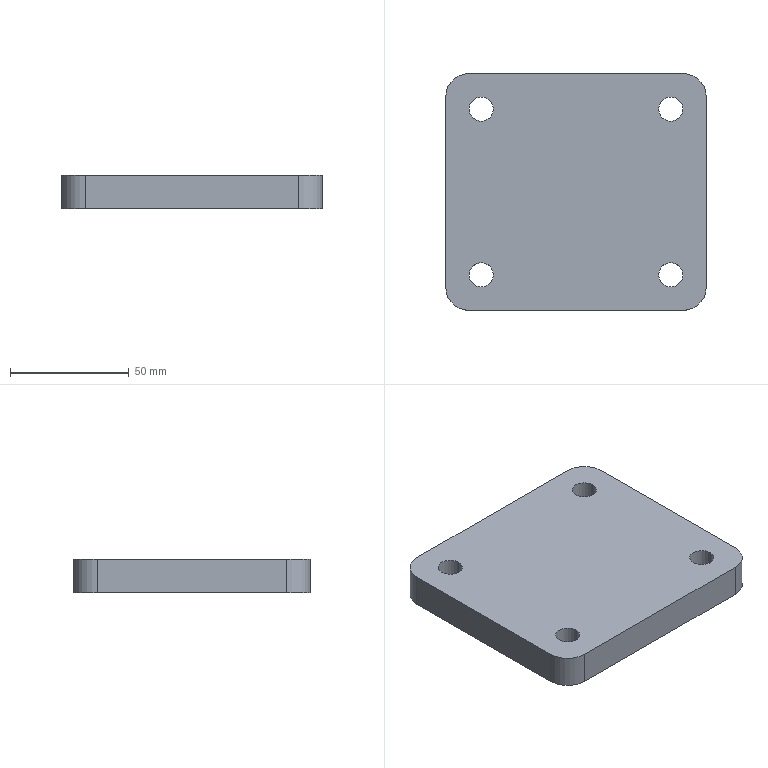Part | SolidWorks | features 3DProfileFeature 1, Extrusion 1, HoleWzd 1 | 1 solid | 18 faces | box 110 x 100 x 14 mm | volume 148222 mm3 | cylinder 12 | plane 6 | commonest cylinder face diameters 10.2 x8 20 x4
STEP:
#1=CARTESIAN_POINT('',(20.1,85.,0.));
#2=VERTEX_POINT('',#1);
#3=CARTESIAN_POINT('',(9.9,85.,0.));
#4=VERTEX_POINT('',#3);
#5=CARTESIAN_POINT('',(15.,85.,0.));
#6=DIRECTION('',(0.,0.,-1.));
#7=DIRECTION('',(-1.,0.,0.));
#8=AXIS2_PLACEMENT_3D('',#5,#6,#7);
#9=CIRCLE('',#8,5.1);
#10=EDGE_CURVE('',#2,#4,#9,.T.);
#11=ORIENTED_EDGE('',*,*,#10,.T.);
#12=CARTESIAN_POINT('',(9.9,85.,14.));
#13=VERTEX_POINT('',#12);
#14=CARTESIAN_POINT('',(9.9,85.,14.));
#15=DIRECTION('',(0.,0.,1.));
#16=VECTOR('',#15,1000.);
#17=LINE('',#14,#16);
#18=EDGE_CURVE('',#4,#13,#17,.T.);
#19=ORIENTED_EDGE('',*,*,#18,.T.);
#20=CARTESIAN_POINT('',(20.1,85.,14.));
#21=VERTEX_POINT('',#20);
#22=CARTESIAN_POINT('',(15.,85.,14.));
#23=DIRECTION('',(0.,0.,1.));
#24=DIRECTION('',(1.,0.,0.));
#25=AXIS2_PLACEMENT_3D('',#22,#23,#24);
#26=CIRCLE('',#25,5.1);
#27=EDGE_CURVE('',#13,#21,#26,.T.);
#28=ORIENTED_EDGE('',*,*,#27,.T.);
#29=CARTESIAN_POINT('',(20.1,85.,14.));
#30=DIRECTION('',(0.,0.,1.));
#31=VECTOR('',#30,1000.);
#32=LINE('',#29,#31);
#33=EDGE_CURVE('',#2,#21,#32,.T.);
#34=ORIENTED_EDGE('',*,*,#33,.F.);
#35=EDGE_LOOP('',(#11,#19,#28,#34));
#36=FACE_OUTER_BOUND('',#35,.T.);
#37=CARTESIAN_POINT('',(15.,85.,14.));
#38=DIRECTION('',(0.,0.,1.));
#39=DIRECTION('',(1.,0.,0.));
#40=AXIS2_PLACEMENT_3D('',#37,#38,#39);
#41=CYLINDRICAL_SURFACE('',#40,5.1);
#42=ADVANCED_FACE('',(#36),#41,.F.);
#43=CARTESIAN_POINT('',(100.1,85.,0.));
#44=VERTEX_POINT('',#43);
#45=CARTESIAN_POINT('',(89.9,85.,0.));
#46=VERTEX_POINT('',#45);
#47=CARTESIAN_POINT('',(95.,85.,0.));
#48=DIRECTION('',(0.,0.,-1.));
#49=DIRECTION('',(-1.,0.,0.));
#50=AXIS2_PLACEMENT_3D('',#47,#48,#49);
#51=CIRCLE('',#50,5.1);
#52=EDGE_CURVE('',#44,#46,#51,.T.);
#53=ORIENTED_EDGE('',*,*,#52,.T.);
#54=CARTESIAN_POINT('',(89.9,85.,14.));
#55=VERTEX_POINT('',#54);
#56=CARTESIAN_POINT('',(89.9,85.,14.));
#57=DIRECTION('',(0.,0.,1.));
#58=VECTOR('',#57,1000.);
#59=LINE('',#56,#58);
#60=EDGE_CURVE('',#46,#55,#59,.T.);
#61=ORIENTED_EDGE('',*,*,#60,.T.);
#62=CARTESIAN_POINT('',(100.1,85.,14.));
#63=VERTEX_POINT('',#62);
#64=CARTESIAN_POINT('',(95.,85.,14.));
#65=DIRECTION('',(0.,0.,1.));
#66=DIRECTION('',(1.,0.,0.));
#67=AXIS2_PLACEMENT_3D('',#64,#65,#66);
#68=CIRCLE('',#67,5.1);
#69=EDGE_CURVE('',#55,#63,#68,.T.);
#70=ORIENTED_EDGE('',*,*,#69,.T.);
#71=CARTESIAN_POINT('',(100.1,85.,14.));
#72=DIRECTION('',(0.,0.,1.));
#73=VECTOR('',#72,1000.);
#74=LINE('',#71,#73);
#75=EDGE_CURVE('',#44,#63,#74,.T.);
#76=ORIENTED_EDGE('',*,*,#75,.F.);
#77=EDGE_LOOP('',(#53,#61,#70,#76));
#78=FACE_OUTER_BOUND('',#77,.T.);
#79=CARTESIAN_POINT('',(95.,85.,14.));
#80=DIRECTION('',(0.,0.,1.));
#81=DIRECTION('',(1.,0.,0.));
#82=AXIS2_PLACEMENT_3D('',#79,#80,#81);
#83=CYLINDRICAL_SURFACE('',#82,5.1);
#84=ADVANCED_FACE('',(#78),#83,.F.);
#85=CARTESIAN_POINT('',(100.1,15.,0.));
#86=VERTEX_POINT('',#85);
#87=CARTESIAN_POINT('',(89.9,15.,0.));
#88=VERTEX_POINT('',#87);
#89=CARTESIAN_POINT('',(95.,15.,0.));
#90=DIRECTION('',(0.,0.,-1.));
#91=DIRECTION('',(-1.,0.,0.));
#92=AXIS2_PLACEMENT_3D('',#89,#90,#91);
#93=CIRCLE('',#92,5.1);
#94=EDGE_CURVE('',#86,#88,#93,.T.);
#95=ORIENTED_EDGE('',*,*,#94,.T.);
#96=CARTESIAN_POINT('',(89.9,15.,14.));
#97=VERTEX_POINT('',#96);
#98=CARTESIAN_POINT('',(89.9,15.,14.));
#99=DIRECTION('',(0.,0.,1.));
#100=VECTOR('',#99,1000.);
#101=LINE('',#98,#100);
#102=EDGE_CURVE('',#88,#97,#101,.T.);
#103=ORIENTED_EDGE('',*,*,#102,.T.);
#104=CARTESIAN_POINT('',(100.1,15.,14.));
#105=VERTEX_POINT('',#104);
#106=CARTESIAN_POINT('',(95.,15.,14.));
#107=DIRECTION('',(0.,0.,1.));
#108=DIRECTION('',(1.,0.,0.));
#109=AXIS2_PLACEMENT_3D('',#106,#107,#108);
#110=CIRCLE('',#109,5.1);
#111=EDGE_CURVE('',#97,#105,#110,.T.);
#112=ORIENTED_EDGE('',*,*,#111,.T.);
#113=CARTESIAN_POINT('',(100.1,15.,14.));
#114=DIRECTION('',(0.,0.,1.));
#115=VECTOR('',#114,1000.);
#116=LINE('',#113,#115);
#117=EDGE_CURVE('',#86,#105,#116,.T.);
#118=ORIENTED_EDGE('',*,*,#117,.F.);
#119=EDGE_LOOP('',(#95,#103,#112,#118));
#120=FACE_OUTER_BOUND('',#119,.T.);
#121=CARTESIAN_POINT('',(95.,15.,14.));
#122=DIRECTION('',(0.,0.,1.));
#123=DIRECTION('',(1.,0.,0.));
#124=AXIS2_PLACEMENT_3D('',#121,#122,#123);
#125=CYLINDRICAL_SURFACE('',#124,5.1);
#126=ADVANCED_FACE('',(#120),#125,.F.);
#127=CARTESIAN_POINT('',(20.1,15.,0.));
#128=VERTEX_POINT('',#127);
#129=CARTESIAN_POINT('',(9.9,15.,0.));
#130=VERTEX_POINT('',#129);
#131=CARTESIAN_POINT('',(15.,15.,0.));
#132=DIRECTION('',(0.,0.,-1.));
#133=DIRECTION('',(-1.,0.,0.));
#134=AXIS2_PLACEMENT_3D('',#131,#132,#133);
#135=CIRCLE('',#134,5.1);
#136=EDGE_CURVE('',#128,#130,#135,.T.);
#137=ORIENTED_EDGE('',*,*,#136,.T.);
#138=CARTESIAN_POINT('',(9.9,15.,14.));
#139=VERTEX_POINT('',#138);
#140=CARTESIAN_POINT('',(9.9,15.,14.));
#141=DIRECTION('',(0.,0.,1.));
#142=VECTOR('',#141,1000.);
#143=LINE('',#140,#142);
#144=EDGE_CURVE('',#130,#139,#143,.T.);
#145=ORIENTED_EDGE('',*,*,#144,.T.);
#146=CARTESIAN_POINT('',(20.1,15.,14.));
#147=VERTEX_POINT('',#146);
#148=CARTESIAN_POINT('',(15.,15.,14.));
#149=DIRECTION('',(0.,0.,1.));
#150=DIRECTION('',(1.,0.,0.));
#151=AXIS2_PLACEMENT_3D('',#148,#149,#150);
#152=CIRCLE('',#151,5.1);
#153=EDGE_CURVE('',#139,#147,#152,.T.);
#154=ORIENTED_EDGE('',*,*,#153,.T.);
#155=CARTESIAN_POINT('',(20.1,15.,14.));
#156=DIRECTION('',(0.,0.,1.));
#157=VECTOR('',#156,1000.);
#158=LINE('',#155,#157);
#159=EDGE_CURVE('',#128,#147,#158,.T.);
#160=ORIENTED_EDGE('',*,*,#159,.F.);
#161=EDGE_LOOP('',(#137,#145,#154,#160));
#162=FACE_OUTER_BOUND('',#161,.T.);
#163=CARTESIAN_POINT('',(15.,15.,14.));
#164=DIRECTION('',(0.,0.,1.));
#165=DIRECTION('',(1.,0.,0.));
#166=AXIS2_PLACEMENT_3D('',#163,#164,#165);
#167=CYLINDRICAL_SURFACE('',#166,5.1);
#168=ADVANCED_FACE('',(#162),#167,.F.);
#169=CARTESIAN_POINT('',(0.,10.,0.));
#170=VERTEX_POINT('',#169);
#171=CARTESIAN_POINT('',(10.,0.,0.));
#172=VERTEX_POINT('',#171);
#173=CARTESIAN_POINT('',(10.,10.,0.));
#174=DIRECTION('',(0.,0.,1.));
#175=DIRECTION('',(-1.,0.,0.));
#176=AXIS2_PLACEMENT_3D('',#173,#174,#175);
#177=CIRCLE('',#176,10.);
#178=EDGE_CURVE('',#170,#172,#177,.T.);
#179=ORIENTED_EDGE('',*,*,#178,.T.);
#180=CARTESIAN_POINT('',(10.,0.,14.));
#181=VERTEX_POINT('',#180);
#182=CARTESIAN_POINT('',(10.,0.,14.));
#183=DIRECTION('',(0.,0.,-1.));
#184=VECTOR('',#183,1000.);
#185=LINE('',#182,#184);
#186=EDGE_CURVE('',#181,#172,#185,.T.);
#187=ORIENTED_EDGE('',*,*,#186,.F.);
#188=CARTESIAN_POINT('',(0.,10.,14.));
#189=VERTEX_POINT('',#188);
#190=CARTESIAN_POINT('',(10.,10.,14.));
#191=DIRECTION('',(0.,0.,1.));
#192=DIRECTION('',(-1.,0.,0.));
#193=AXIS2_PLACEMENT_3D('',#190,#191,#192);
#194=CIRCLE('',#193,10.);
#195=EDGE_CURVE('',#189,#181,#194,.T.);
#196=ORIENTED_EDGE('',*,*,#195,.F.);
#197=CARTESIAN_POINT('',(0.,10.,14.));
#198=DIRECTION('',(0.,0.,-1.));
#199=VECTOR('',#198,1000.);
#200=LINE('',#197,#199);
#201=EDGE_CURVE('',#189,#170,#200,.T.);
#202=ORIENTED_EDGE('',*,*,#201,.T.);
#203=EDGE_LOOP('',(#179,#187,#196,#202));
#204=FACE_OUTER_BOUND('',#203,.T.);
#205=CARTESIAN_POINT('',(10.,10.,14.));
#206=DIRECTION('',(0.,0.,-1.));
#207=DIRECTION('',(-1.,0.,0.));
#208=AXIS2_PLACEMENT_3D('',#205,#206,#207);
#209=CYLINDRICAL_SURFACE('',#208,10.);
#210=ADVANCED_FACE('',(#204),#209,.T.);
#211=CARTESIAN_POINT('',(100.,0.,0.));
#212=VERTEX_POINT('',#211);
#213=CARTESIAN_POINT('',(10.,0.,0.));
#214=DIRECTION('',(1.,0.,0.));
#215=VECTOR('',#214,1000.);
#216=LINE('',#213,#215);
#217=EDGE_CURVE('',#172,#212,#216,.T.);
#218=ORIENTED_EDGE('',*,*,#217,.T.);
#219=CARTESIAN_POINT('',(100.,0.,14.));
#220=VERTEX_POINT('',#219);
#221=CARTESIAN_POINT('',(100.,0.,14.));
#222=DIRECTION('',(0.,0.,-1.));
#223=VECTOR('',#222,1000.);
#224=LINE('',#221,#223);
#225=EDGE_CURVE('',#220,#212,#224,.T.);
#226=ORIENTED_EDGE('',*,*,#225,.F.);
#227=CARTESIAN_POINT('',(10.,0.,14.));
#228=DIRECTION('',(1.,0.,0.));
#229=VECTOR('',#228,1000.);
#230=LINE('',#227,#229);
#231=EDGE_CURVE('',#181,#220,#230,.T.);
#232=ORIENTED_EDGE('',*,*,#231,.F.);
#233=ORIENTED_EDGE('',*,*,#186,.T.);
#234=EDGE_LOOP('',(#218,#226,#232,#233));
#235=FACE_OUTER_BOUND('',#234,.T.);
#236=CARTESIAN_POINT('',(10.,0.,14.));
#237=DIRECTION('',(0.,1.,0.));
#238=DIRECTION('',(0.,0.,1.));
#239=AXIS2_PLACEMENT_3D('',#236,#237,#238);
#240=PLANE('',#239);
#241=ADVANCED_FACE('',(#235),#240,.F.);
#242=CARTESIAN_POINT('',(110.,10.,0.));
#243=VERTEX_POINT('',#242);
#244=CARTESIAN_POINT('',(100.,10.,0.));
#245=DIRECTION('',(0.,0.,1.));
#246=DIRECTION('',(1.,0.,0.));
#247=AXIS2_PLACEMENT_3D('',#244,#245,#246);
#248=CIRCLE('',#247,10.);
#249=EDGE_CURVE('',#212,#243,#248,.T.);
#250=ORIENTED_EDGE('',*,*,#249,.T.);
#251=CARTESIAN_POINT('',(110.,10.,14.));
#252=VERTEX_POINT('',#251);
#253=CARTESIAN_POINT('',(110.,10.,14.));
#254=DIRECTION('',(0.,0.,-1.));
#255=VECTOR('',#254,1000.);
#256=LINE('',#253,#255);
#257=EDGE_CURVE('',#252,#243,#256,.T.);
#258=ORIENTED_EDGE('',*,*,#257,.F.);
#259=CARTESIAN_POINT('',(100.,10.,14.));
#260=DIRECTION('',(0.,0.,1.));
#261=DIRECTION('',(1.,0.,0.));
#262=AXIS2_PLACEMENT_3D('',#259,#260,#261);
#263=CIRCLE('',#262,10.);
#264=EDGE_CURVE('',#220,#252,#263,.T.);
#265=ORIENTED_EDGE('',*,*,#264,.F.);
#266=ORIENTED_EDGE('',*,*,#225,.T.);
#267=EDGE_LOOP('',(#250,#258,#265,#266));
#268=FACE_OUTER_BOUND('',#267,.T.);
#269=CARTESIAN_POINT('',(100.,10.,14.));
#270=DIRECTION('',(0.,0.,-1.));
#271=DIRECTION('',(-1.,0.,0.));
#272=AXIS2_PLACEMENT_3D('',#269,#270,#271);
#273=CYLINDRICAL_SURFACE('',#272,10.);
#274=ADVANCED_FACE('',(#268),#273,.T.);
#275=CARTESIAN_POINT('',(110.,90.,0.));
#276=VERTEX_POINT('',#275);
#277=CARTESIAN_POINT('',(110.,10.,0.));
#278=DIRECTION('',(0.,1.,0.));
#279=VECTOR('',#278,1000.);
#280=LINE('',#277,#279);
#281=EDGE_CURVE('',#243,#276,#280,.T.);
#282=ORIENTED_EDGE('',*,*,#281,.T.);
#283=CARTESIAN_POINT('',(110.,90.,14.));
#284=VERTEX_POINT('',#283);
#285=CARTESIAN_POINT('',(110.,90.,14.));
#286=DIRECTION('',(0.,0.,-1.));
#287=VECTOR('',#286,1000.);
#288=LINE('',#285,#287);
#289=EDGE_CURVE('',#284,#276,#288,.T.);
#290=ORIENTED_EDGE('',*,*,#289,.F.);
#291=CARTESIAN_POINT('',(110.,10.,14.));
#292=DIRECTION('',(0.,1.,0.));
#293=VECTOR('',#292,1000.);
#294=LINE('',#291,#293);
#295=EDGE_CURVE('',#252,#284,#294,.T.);
#296=ORIENTED_EDGE('',*,*,#295,.F.);
#297=ORIENTED_EDGE('',*,*,#257,.T.);
#298=EDGE_LOOP('',(#282,#290,#296,#297));
#299=FACE_OUTER_BOUND('',#298,.T.);
#300=CARTESIAN_POINT('',(110.,10.,14.));
#301=DIRECTION('',(-1.,0.,0.));
#302=DIRECTION('',(0.,0.,1.));
#303=AXIS2_PLACEMENT_3D('',#300,#301,#302);
#304=PLANE('',#303);
#305=ADVANCED_FACE('',(#299),#304,.F.);
#306=CARTESIAN_POINT('',(100.,100.,0.));
#307=VERTEX_POINT('',#306);
#308=CARTESIAN_POINT('',(100.,90.,0.));
#309=DIRECTION('',(0.,0.,1.));
#310=DIRECTION('',(-1.,0.,0.));
#311=AXIS2_PLACEMENT_3D('',#308,#309,#310);
#312=CIRCLE('',#311,10.);
#313=EDGE_CURVE('',#276,#307,#312,.T.);
#314=ORIENTED_EDGE('',*,*,#313,.T.);
#315=CARTESIAN_POINT('',(100.,100.,14.));
#316=VERTEX_POINT('',#315);
#317=CARTESIAN_POINT('',(100.,100.,14.));
#318=DIRECTION('',(0.,0.,-1.));
#319=VECTOR('',#318,1000.);
#320=LINE('',#317,#319);
#321=EDGE_CURVE('',#316,#307,#320,.T.);
#322=ORIENTED_EDGE('',*,*,#321,.F.);
#323=CARTESIAN_POINT('',(100.,90.,14.));
#324=DIRECTION('',(0.,0.,1.));
#325=DIRECTION('',(-1.,0.,0.));
#326=AXIS2_PLACEMENT_3D('',#323,#324,#325);
#327=CIRCLE('',#326,10.);
#328=EDGE_CURVE('',#284,#316,#327,.T.);
#329=ORIENTED_EDGE('',*,*,#328,.F.);
#330=ORIENTED_EDGE('',*,*,#289,.T.);
#331=EDGE_LOOP('',(#314,#322,#329,#330));
#332=FACE_OUTER_BOUND('',#331,.T.);
#333=CARTESIAN_POINT('',(100.,90.,14.));
#334=DIRECTION('',(0.,0.,-1.));
#335=DIRECTION('',(-1.,0.,0.));
#336=AXIS2_PLACEMENT_3D('',#333,#334,#335);
#337=CYLINDRICAL_SURFACE('',#336,10.);
#338=ADVANCED_FACE('',(#332),#337,.T.);
#339=CARTESIAN_POINT('',(10.,100.,0.));
#340=VERTEX_POINT('',#339);
#341=CARTESIAN_POINT('',(10.,100.,0.));
#342=DIRECTION('',(-1.,0.,0.));
#343=VECTOR('',#342,1000.);
#344=LINE('',#341,#343);
#345=EDGE_CURVE('',#307,#340,#344,.T.);
#346=ORIENTED_EDGE('',*,*,#345,.T.);
#347=CARTESIAN_POINT('',(10.,100.,14.));
#348=VERTEX_POINT('',#347);
#349=CARTESIAN_POINT('',(10.,100.,14.));
#350=DIRECTION('',(0.,0.,-1.));
#351=VECTOR('',#350,1000.);
#352=LINE('',#349,#351);
#353=EDGE_CURVE('',#348,#340,#352,.T.);
#354=ORIENTED_EDGE('',*,*,#353,.F.);
#355=CARTESIAN_POINT('',(10.,100.,14.));
#356=DIRECTION('',(-1.,0.,0.));
#357=VECTOR('',#356,1000.);
#358=LINE('',#355,#357);
#359=EDGE_CURVE('',#316,#348,#358,.T.);
#360=ORIENTED_EDGE('',*,*,#359,.F.);
#361=ORIENTED_EDGE('',*,*,#321,.T.);
#362=EDGE_LOOP('',(#346,#354,#360,#361));
#363=FACE_OUTER_BOUND('',#362,.T.);
#364=CARTESIAN_POINT('',(10.,100.,14.));
#365=DIRECTION('',(0.,-1.,0.));
#366=DIRECTION('',(0.,0.,-1.));
#367=AXIS2_PLACEMENT_3D('',#364,#365,#366);
#368=PLANE('',#367);
#369=ADVANCED_FACE('',(#363),#368,.F.);
#370=CARTESIAN_POINT('',(0.,90.,0.));
#371=VERTEX_POINT('',#370);
#372=CARTESIAN_POINT('',(10.,90.,0.));
#373=DIRECTION('',(0.,0.,1.));
#374=DIRECTION('',(-1.,0.,0.));
#375=AXIS2_PLACEMENT_3D('',#372,#373,#374);
#376=CIRCLE('',#375,10.);
#377=EDGE_CURVE('',#340,#371,#376,.T.);
#378=ORIENTED_EDGE('',*,*,#377,.T.);
#379=CARTESIAN_POINT('',(0.,90.,14.));
#380=VERTEX_POINT('',#379);
#381=CARTESIAN_POINT('',(0.,90.,14.));
#382=DIRECTION('',(0.,0.,-1.));
#383=VECTOR('',#382,1000.);
#384=LINE('',#381,#383);
#385=EDGE_CURVE('',#380,#371,#384,.T.);
#386=ORIENTED_EDGE('',*,*,#385,.F.);
#387=CARTESIAN_POINT('',(10.,90.,14.));
#388=DIRECTION('',(0.,0.,1.));
#389=DIRECTION('',(-1.,0.,0.));
#390=AXIS2_PLACEMENT_3D('',#387,#388,#389);
#391=CIRCLE('',#390,10.);
#392=EDGE_CURVE('',#348,#380,#391,.T.);
#393=ORIENTED_EDGE('',*,*,#392,.F.);
#394=ORIENTED_EDGE('',*,*,#353,.T.);
#395=EDGE_LOOP('',(#378,#386,#393,#394));
#396=FACE_OUTER_BOUND('',#395,.T.);
#397=CARTESIAN_POINT('',(10.,90.,14.));
#398=DIRECTION('',(0.,0.,-1.));
#399=DIRECTION('',(-1.,0.,0.));
#400=AXIS2_PLACEMENT_3D('',#397,#398,#399);
#401=CYLINDRICAL_SURFACE('',#400,10.);
#402=ADVANCED_FACE('',(#396),#401,.T.);
#403=CARTESIAN_POINT('',(0.,10.,0.));
#404=DIRECTION('',(0.,-1.,0.));
#405=VECTOR('',#404,1000.);
#406=LINE('',#403,#405);
#407=EDGE_CURVE('',#371,#170,#406,.T.);
#408=ORIENTED_EDGE('',*,*,#407,.T.);
#409=ORIENTED_EDGE('',*,*,#201,.F.);
#410=CARTESIAN_POINT('',(0.,10.,14.));
#411=DIRECTION('',(0.,-1.,0.));
#412=VECTOR('',#411,1000.);
#413=LINE('',#410,#412);
#414=EDGE_CURVE('',#380,#189,#413,.T.);
#415=ORIENTED_EDGE('',*,*,#414,.F.);
#416=ORIENTED_EDGE('',*,*,#385,.T.);
#417=EDGE_LOOP('',(#408,#409,#415,#416));
#418=FACE_OUTER_BOUND('',#417,.T.);
#419=CARTESIAN_POINT('',(0.,10.,14.));
#420=DIRECTION('',(1.,0.,0.));
#421=DIRECTION('',(0.,0.,-1.));
#422=AXIS2_PLACEMENT_3D('',#419,#420,#421);
#423=PLANE('',#422);
#424=ADVANCED_FACE('',(#418),#423,.F.);
#425=CARTESIAN_POINT('',(15.,85.,14.));
#426=DIRECTION('',(0.,0.,1.));
#427=DIRECTION('',(1.,0.,0.));
#428=AXIS2_PLACEMENT_3D('',#425,#426,#427);
#429=CIRCLE('',#428,5.1);
#430=EDGE_CURVE('',#21,#13,#429,.T.);
#431=ORIENTED_EDGE('',*,*,#430,.F.);
#432=ORIENTED_EDGE('',*,*,#27,.F.);
#433=EDGE_LOOP('',(#431,#432));
#434=FACE_BOUND('',#433,.T.);
#435=CARTESIAN_POINT('',(95.,85.,14.));
#436=DIRECTION('',(0.,0.,1.));
#437=DIRECTION('',(1.,0.,0.));
#438=AXIS2_PLACEMENT_3D('',#435,#436,#437);
#439=CIRCLE('',#438,5.1);
#440=EDGE_CURVE('',#63,#55,#439,.T.);
#441=ORIENTED_EDGE('',*,*,#440,.F.);
#442=ORIENTED_EDGE('',*,*,#69,.F.);
#443=EDGE_LOOP('',(#441,#442));
#444=FACE_BOUND('',#443,.T.);
#445=CARTESIAN_POINT('',(95.,15.,14.));
#446=DIRECTION('',(0.,0.,1.));
#447=DIRECTION('',(1.,0.,0.));
#448=AXIS2_PLACEMENT_3D('',#445,#446,#447);
#449=CIRCLE('',#448,5.1);
#450=EDGE_CURVE('',#105,#97,#449,.T.);
#451=ORIENTED_EDGE('',*,*,#450,.F.);
#452=ORIENTED_EDGE('',*,*,#111,.F.);
#453=EDGE_LOOP('',(#451,#452));
#454=FACE_BOUND('',#453,.T.);
#455=CARTESIAN_POINT('',(15.,15.,14.));
#456=DIRECTION('',(0.,0.,1.));
#457=DIRECTION('',(1.,0.,0.));
#458=AXIS2_PLACEMENT_3D('',#455,#456,#457);
#459=CIRCLE('',#458,5.1);
#460=EDGE_CURVE('',#147,#139,#459,.T.);
#461=ORIENTED_EDGE('',*,*,#460,.F.);
#462=ORIENTED_EDGE('',*,*,#153,.F.);
#463=EDGE_LOOP('',(#461,#462));
#464=FACE_BOUND('',#463,.T.);
#465=ORIENTED_EDGE('',*,*,#195,.T.);
#466=ORIENTED_EDGE('',*,*,#231,.T.);
#467=ORIENTED_EDGE('',*,*,#264,.T.);
#468=ORIENTED_EDGE('',*,*,#295,.T.);
#469=ORIENTED_EDGE('',*,*,#328,.T.);
#470=ORIENTED_EDGE('',*,*,#359,.T.);
#471=ORIENTED_EDGE('',*,*,#392,.T.);
#472=ORIENTED_EDGE('',*,*,#414,.T.);
#473=EDGE_LOOP('',(#465,#466,#467,#468,#469,#470,#471,#472));
#474=FACE_OUTER_BOUND('',#473,.T.);
#475=CARTESIAN_POINT('',(10.,10.,14.));
#476=DIRECTION('',(0.,0.,-1.));
#477=DIRECTION('',(-1.,0.,0.));
#478=AXIS2_PLACEMENT_3D('',#475,#476,#477);
#479=PLANE('',#478);
#480=ADVANCED_FACE('',(#434,#444,#454,#464,#474),#479,.F.);
#481=ORIENTED_EDGE('',*,*,#10,.F.);
#482=CARTESIAN_POINT('',(15.,85.,0.));
#483=DIRECTION('',(0.,0.,-1.));
#484=DIRECTION('',(-1.,0.,0.));
#485=AXIS2_PLACEMENT_3D('',#482,#483,#484);
#486=CIRCLE('',#485,5.1);
#487=EDGE_CURVE('',#4,#2,#486,.T.);
#488=ORIENTED_EDGE('',*,*,#487,.F.);
#489=EDGE_LOOP('',(#481,#488));
#490=FACE_BOUND('',#489,.T.);
#491=ORIENTED_EDGE('',*,*,#52,.F.);
#492=CARTESIAN_POINT('',(95.,85.,0.));
#493=DIRECTION('',(0.,0.,-1.));
#494=DIRECTION('',(-1.,0.,0.));
#495=AXIS2_PLACEMENT_3D('',#492,#493,#494);
#496=CIRCLE('',#495,5.1);
#497=EDGE_CURVE('',#46,#44,#496,.T.);
#498=ORIENTED_EDGE('',*,*,#497,.F.);
#499=EDGE_LOOP('',(#491,#498));
#500=FACE_BOUND('',#499,.T.);
#501=ORIENTED_EDGE('',*,*,#94,.F.);
#502=CARTESIAN_POINT('',(95.,15.,0.));
#503=DIRECTION('',(0.,0.,-1.));
#504=DIRECTION('',(-1.,0.,0.));
#505=AXIS2_PLACEMENT_3D('',#502,#503,#504);
#506=CIRCLE('',#505,5.1);
#507=EDGE_CURVE('',#88,#86,#506,.T.);
#508=ORIENTED_EDGE('',*,*,#507,.F.);
#509=EDGE_LOOP('',(#501,#508));
#510=FACE_BOUND('',#509,.T.);
#511=ORIENTED_EDGE('',*,*,#136,.F.);
#512=CARTESIAN_POINT('',(15.,15.,0.));
#513=DIRECTION('',(0.,0.,-1.));
#514=DIRECTION('',(-1.,0.,0.));
#515=AXIS2_PLACEMENT_3D('',#512,#513,#514);
#516=CIRCLE('',#515,5.1);
#517=EDGE_CURVE('',#130,#128,#516,.T.);
#518=ORIENTED_EDGE('',*,*,#517,.F.);
#519=EDGE_LOOP('',(#511,#518));
#520=FACE_BOUND('',#519,.T.);
#521=ORIENTED_EDGE('',*,*,#178,.F.);
#522=ORIENTED_EDGE('',*,*,#407,.F.);
#523=ORIENTED_EDGE('',*,*,#377,.F.);
#524=ORIENTED_EDGE('',*,*,#345,.F.);
#525=ORIENTED_EDGE('',*,*,#313,.F.);
#526=ORIENTED_EDGE('',*,*,#281,.F.);
#527=ORIENTED_EDGE('',*,*,#249,.F.);
#528=ORIENTED_EDGE('',*,*,#217,.F.);
#529=EDGE_LOOP('',(#521,#522,#523,#524,#525,#526,#527,#528));
#530=FACE_OUTER_BOUND('',#529,.T.);
#531=CARTESIAN_POINT('',(10.,10.,0.));
#532=DIRECTION('',(0.,0.,-1.));
#533=DIRECTION('',(-1.,0.,0.));
#534=AXIS2_PLACEMENT_3D('',#531,#532,#533);
#535=PLANE('',#534);
#536=ADVANCED_FACE('',(#490,#500,#510,#520,#530),#535,.T.);
#537=ORIENTED_EDGE('',*,*,#144,.F.);
#538=ORIENTED_EDGE('',*,*,#517,.T.);
#539=ORIENTED_EDGE('',*,*,#159,.T.);
#540=ORIENTED_EDGE('',*,*,#460,.T.);
#541=EDGE_LOOP('',(#537,#538,#539,#540));
#542=FACE_OUTER_BOUND('',#541,.T.);
#543=CARTESIAN_POINT('',(15.,15.,14.));
#544=DIRECTION('',(0.,0.,1.));
#545=DIRECTION('',(1.,0.,0.));
#546=AXIS2_PLACEMENT_3D('',#543,#544,#545);
#547=CYLINDRICAL_SURFACE('',#546,5.1);
#548=ADVANCED_FACE('',(#542),#547,.F.);
#549=ORIENTED_EDGE('',*,*,#102,.F.);
#550=ORIENTED_EDGE('',*,*,#507,.T.);
#551=ORIENTED_EDGE('',*,*,#117,.T.);
#552=ORIENTED_EDGE('',*,*,#450,.T.);
#553=EDGE_LOOP('',(#549,#550,#551,#552));
#554=FACE_OUTER_BOUND('',#553,.T.);
#555=CARTESIAN_POINT('',(95.,15.,14.));
#556=DIRECTION('',(0.,0.,1.));
#557=DIRECTION('',(1.,0.,0.));
#558=AXIS2_PLACEMENT_3D('',#555,#556,#557);
#559=CYLINDRICAL_SURFACE('',#558,5.1);
#560=ADVANCED_FACE('',(#554),#559,.F.);
#561=ORIENTED_EDGE('',*,*,#60,.F.);
#562=ORIENTED_EDGE('',*,*,#497,.T.);
#563=ORIENTED_EDGE('',*,*,#75,.T.);
#564=ORIENTED_EDGE('',*,*,#440,.T.);
#565=EDGE_LOOP('',(#561,#562,#563,#564));
#566=FACE_OUTER_BOUND('',#565,.T.);
#567=CARTESIAN_POINT('',(95.,85.,14.));
#568=DIRECTION('',(0.,0.,1.));
#569=DIRECTION('',(1.,0.,0.));
#570=AXIS2_PLACEMENT_3D('',#567,#568,#569);
#571=CYLINDRICAL_SURFACE('',#570,5.1);
#572=ADVANCED_FACE('',(#566),#571,.F.);
#573=ORIENTED_EDGE('',*,*,#18,.F.);
#574=ORIENTED_EDGE('',*,*,#487,.T.);
#575=ORIENTED_EDGE('',*,*,#33,.T.);
#576=ORIENTED_EDGE('',*,*,#430,.T.);
#577=EDGE_LOOP('',(#573,#574,#575,#576));
#578=FACE_OUTER_BOUND('',#577,.T.);
#579=CARTESIAN_POINT('',(15.,85.,14.));
#580=DIRECTION('',(0.,0.,1.));
#581=DIRECTION('',(1.,0.,0.));
#582=AXIS2_PLACEMENT_3D('',#579,#580,#581);
#583=CYLINDRICAL_SURFACE('',#582,5.1);
#584=ADVANCED_FACE('',(#578),#583,.F.);
#585=CLOSED_SHELL('',(#42,#84,#126,#168,#210,#241,#274,#305,#338,#369,#402,#424,#480,#536,#548,#560,#572,#584));
#586=MANIFOLD_SOLID_BREP('',#585);
#587=CARTESIAN_POINT('',(0.,0.,0.));
#588=DIRECTION('',(0.,0.,1.));
#589=DIRECTION('',(1.,0.,0.));
#590=AXIS2_PLACEMENT_3D('',#587,#588,#589);
#591=(LENGTH_UNIT()NAMED_UNIT(*)SI_UNIT(.MILLI.,.METRE.));
#592=UNCERTAINTY_MEASURE_WITH_UNIT(LENGTH_MEASURE(0.00001),#591,'','');
#593=(NAMED_UNIT(*)PLANE_ANGLE_UNIT()SI_UNIT($,.RADIAN.));
#594=(NAMED_UNIT(*)SI_UNIT($,.STERADIAN.)SOLID_ANGLE_UNIT());
#595=(GEOMETRIC_REPRESENTATION_CONTEXT(3)GLOBAL_UNCERTAINTY_ASSIGNED_CONTEXT((#592))GLOBAL_UNIT_ASSIGNED_CONTEXT((#591,#593,#594))REPRESENTATION_CONTEXT('',''));
#596=ADVANCED_BREP_SHAPE_REPRESENTATION('',(#586,#590),#595);